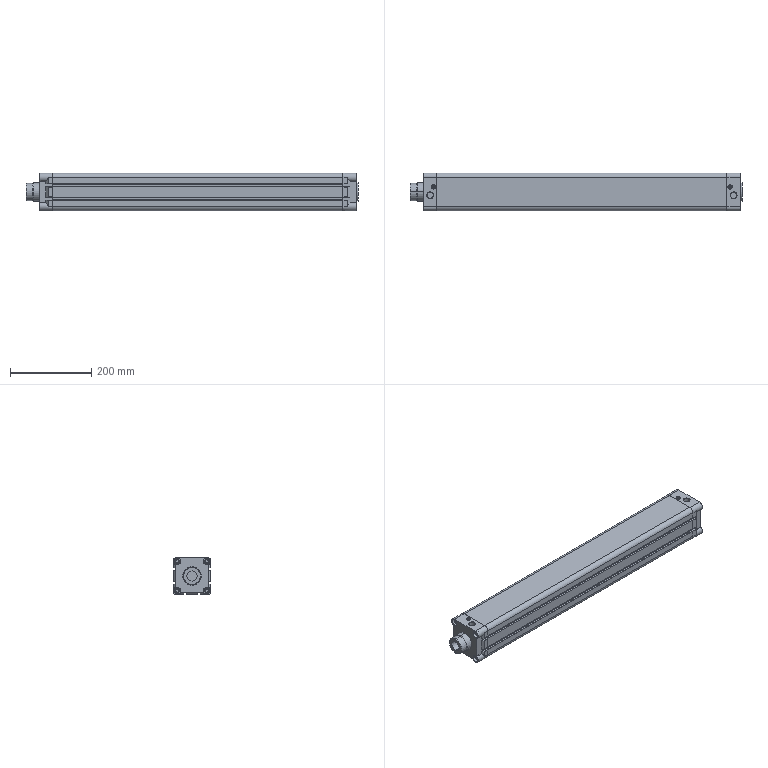Part | NX | features BREP 1 | 1 solid | 398 faces | box 815 x 93 x 93 mm | volume 2861841 mm3 | cylinder 190 | plane 176 | cone 30 | torus 2 | commonest cylinder face diameters 1 x102 8.376 x16 15.9 x16 22 x16 21 x10 5 x4